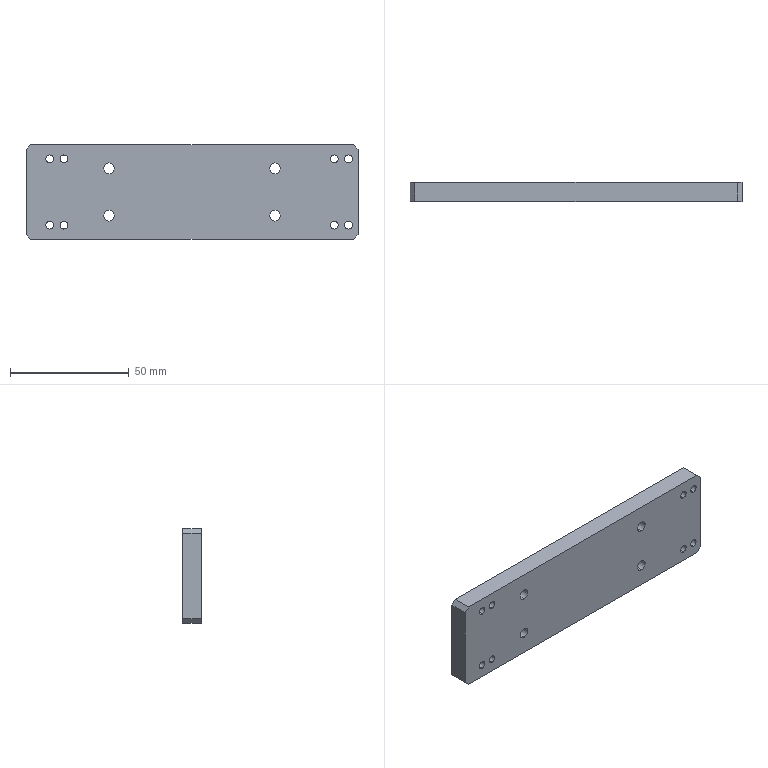Part | STEP file | PN_0039 vibratory feeder connecting plate | 1 solid | 46 faces | box 140 x 8 x 40 mm | volume 43075 mm3 | cylinder 32 | plane 14 | commonest cylinder face diameters 3.3 x16 4.5 x8 8 x8